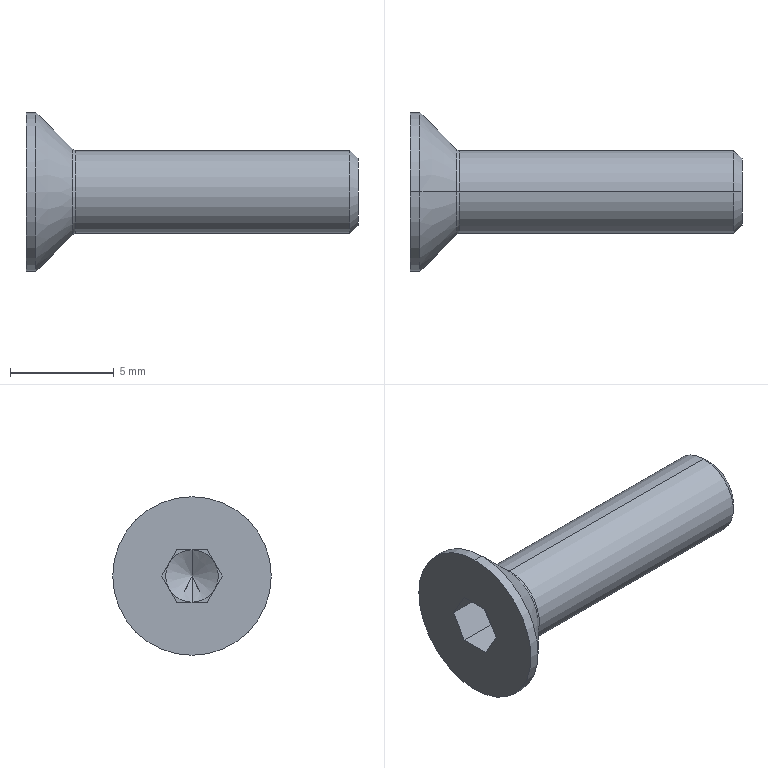Part | STEP file | socket countersunk head screw_din_DIN 7991 - M4 x 16 --- 11.6N | 1 solid | 26 faces | box 16 x 7.64 x 7.64 mm | volume 232.169 mm3 | plane 14 | cone 6 | cylinder 4 | torus 2 | commonest cylinder face diameters 4 x2 7.64 x2